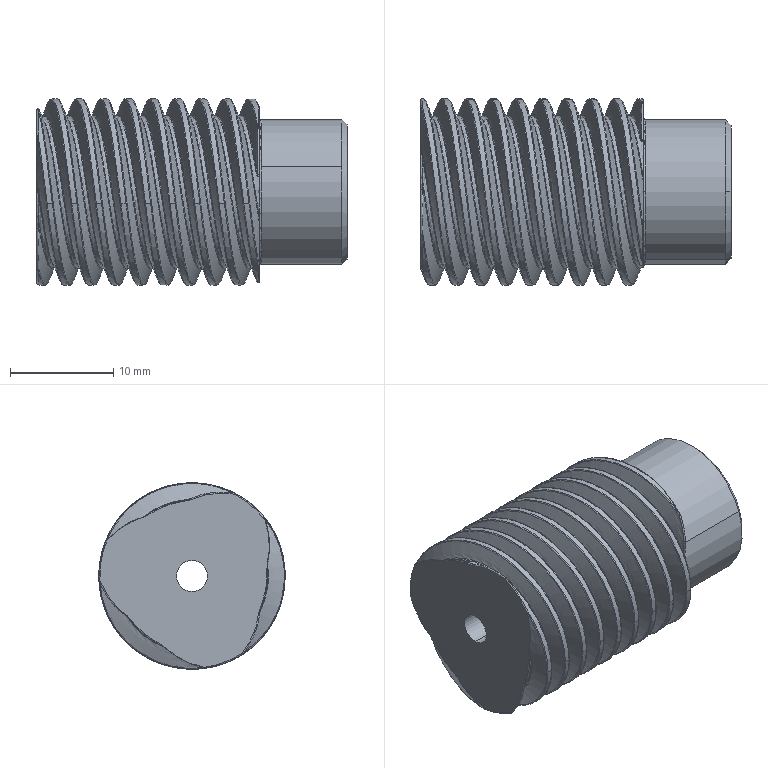Part | SolidWorks | features ICE 3, Chamfer 1, DeleteBody 1, MBimport 1 | 1 solid | 95 faces | box 30 x 18.04 x 18.04 mm | volume 5689 mm3 | spline 42 | cylinder 22 | sphere 18 | torus 8 | plane 3 | cone 2 | commonest cylinder face diameters 18.04 x18 3 x2 14 x2